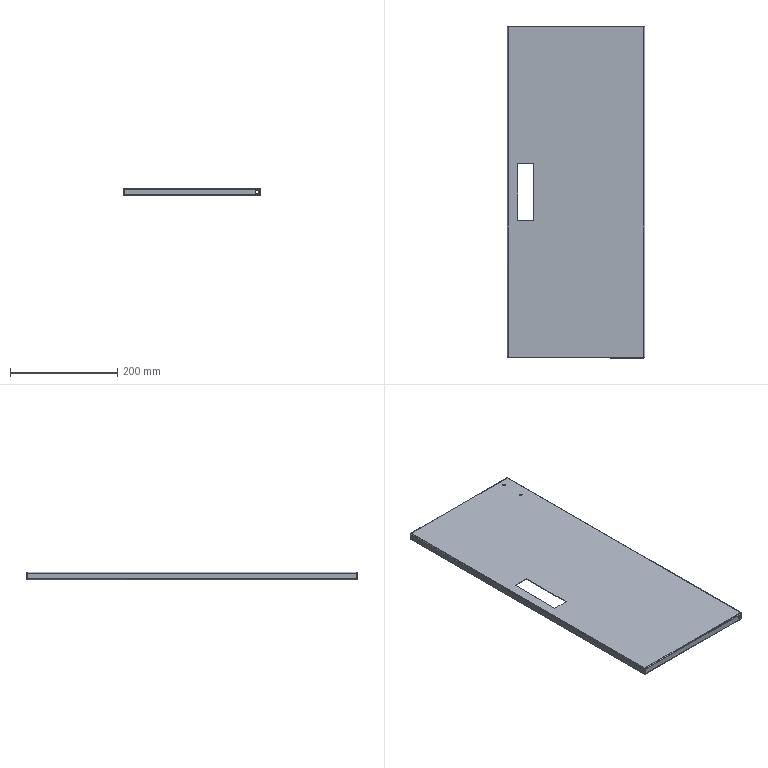Part | SolidWorks | features EdgeFlange 2, ICE 2, SMBaseFlange 2, Cut 1, Fillet 1, FlatPattern 1, LPattern 1, SheetMetal 1 | 1 solid | 90 faces | box 257 x 620 x 14 mm | volume 226694 mm3 | plane 48 | cylinder 26 | spline 16 | commonest cylinder face diameters 1 x4 1.2 x4 3.4 x4 3.6 x4 5 x4 6.3 x4